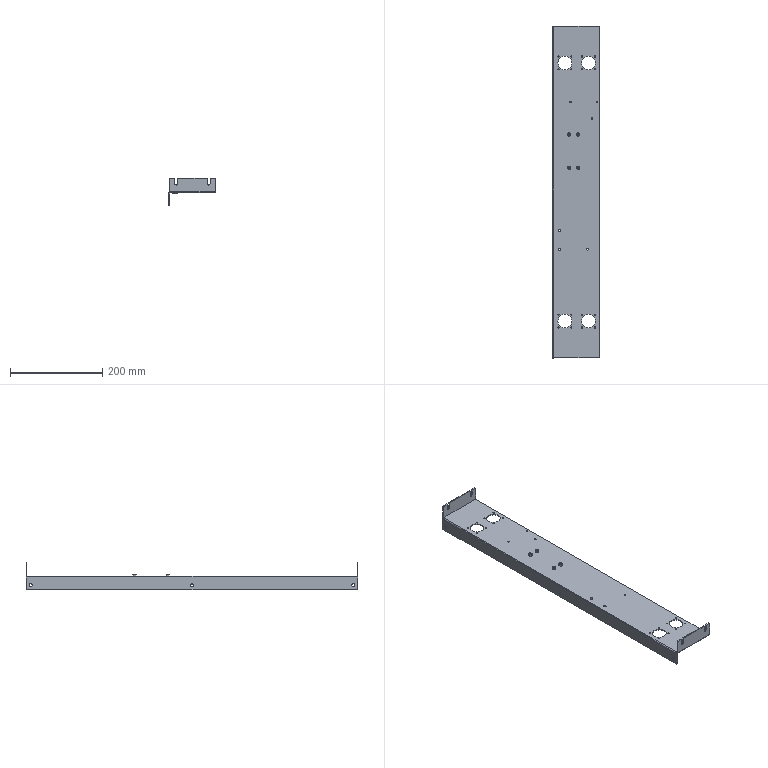Part | STEP file | Power strip mounting plate | 1 solid | 138 faces | box 100 x 719 x 60 mm | volume 188882 mm3 | cylinder 94 | plane 44 | commonest cylinder face diameters 2.5 x32 3.3 x16 7.1 x8 30 x8 4 x6 6.5 x6